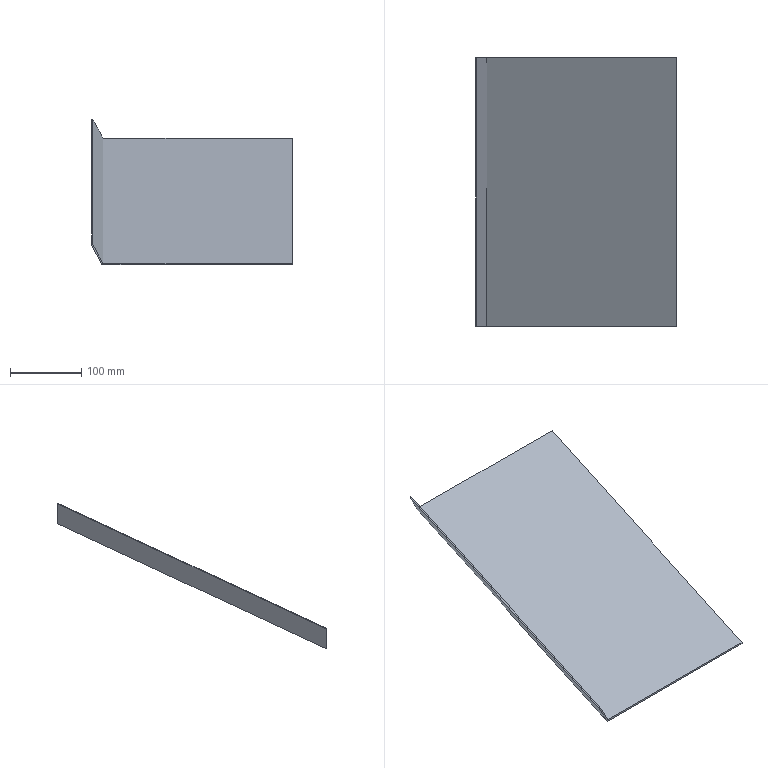Part | NX | features solid 2 | 1 solid | 8 faces | box 281.246 x 376.011 x 204.125 mm | volume 244430 mm3 | plane 8
STEP:
#1=CARTESIAN_POINT('',(748.754,-108.989,-45.166));
#2=VERTEX_POINT('',#1);
#3=CARTESIAN_POINT('',(763.321,-108.989,-73.005));
#4=VERTEX_POINT('',#3);
#5=CARTESIAN_POINT('',(693.858,-108.989,59.746));
#6=DIRECTION('',(0.4636,0.,-0.886));
#7=VECTOR('',#6,1000.);
#8=LINE('',#5,#7);
#9=EDGE_CURVE('',#2,#4,#8,.T.);
#10=ORIENTED_EDGE('',*,*,#9,.F.);
#11=CARTESIAN_POINT('',(750.567,-108.989,-44.218));
#12=VERTEX_POINT('',#11);
#13=CARTESIAN_POINT('',(876.733,-108.989,21.8));
#14=DIRECTION('',(0.886,0.,0.4636));
#15=VECTOR('',#14,1000.);
#16=LINE('',#13,#15);
#17=EDGE_CURVE('',#2,#12,#16,.T.);
#18=ORIENTED_EDGE('',*,*,#17,.T.);
#19=CARTESIAN_POINT('',(764.475,-108.989,-70.799));
#20=VERTEX_POINT('',#19);
#21=CARTESIAN_POINT('',(695.671,-108.989,60.694));
#22=DIRECTION('',(0.4636,0.,-0.886));
#23=VECTOR('',#22,1000.);
#24=LINE('',#21,#23);
#25=EDGE_CURVE('',#12,#20,#24,.T.);
#26=ORIENTED_EDGE('',*,*,#25,.T.);
#27=CARTESIAN_POINT('',(1030.,-108.989,-70.799));
#28=VERTEX_POINT('',#27);
#29=CARTESIAN_POINT('',(930.,-108.989,-70.799));
#30=DIRECTION('',(-1.,0.,0.));
#31=VECTOR('',#30,1000.);
#32=LINE('',#29,#31);
#33=EDGE_CURVE('',#28,#20,#32,.T.);
#34=ORIENTED_EDGE('',*,*,#33,.F.);
#35=CARTESIAN_POINT('',(1030.,-108.989,-73.005));
#36=VERTEX_POINT('',#35);
#37=CARTESIAN_POINT('',(1030.,-108.989,-80.));
#38=DIRECTION('',(0.,0.,1.));
#39=VECTOR('',#38,1000.);
#40=LINE('',#37,#39);
#41=EDGE_CURVE('',#36,#28,#40,.T.);
#42=ORIENTED_EDGE('',*,*,#41,.F.);
#43=CARTESIAN_POINT('',(930.,-108.989,-73.005));
#44=DIRECTION('',(-1.,0.,0.));
#45=VECTOR('',#44,1000.);
#46=LINE('',#43,#45);
#47=EDGE_CURVE('',#36,#4,#46,.T.);
#48=ORIENTED_EDGE('',*,*,#47,.T.);
#49=EDGE_LOOP('',(#10,#18,#26,#34,#42,#48));
#50=FACE_BOUND('',#49,.T.);
#51=CARTESIAN_POINT('',(930.,-108.989,-80.));
#52=DIRECTION('',(0.,-1.,0.));
#53=DIRECTION('',(0.,0.,-1.));
#54=AXIS2_PLACEMENT_3D('',#51,#52,#53);
#55=PLANE('',#54);
#56=ADVANCED_FACE('',(#50),#55,.F.);
#57=ORIENTED_EDGE('',*,*,#47,.F.);
#58=CARTESIAN_POINT('',(1030.,-485.,-248.342));
#59=VERTEX_POINT('',#58);
#60=CARTESIAN_POINT('',(1030.,-511.683,-260.785));
#61=DIRECTION('',(0.,0.9063,0.4226));
#62=VECTOR('',#61,1000.);
#63=LINE('',#60,#62);
#64=EDGE_CURVE('',#59,#36,#63,.T.);
#65=ORIENTED_EDGE('',*,*,#64,.F.);
#66=CARTESIAN_POINT('',(763.321,-485.,-248.342));
#67=VERTEX_POINT('',#66);
#68=CARTESIAN_POINT('',(930.,-485.,-248.342));
#69=DIRECTION('',(1.,0.,0.));
#70=VECTOR('',#69,1000.);
#71=LINE('',#68,#70);
#72=EDGE_CURVE('',#59,#67,#71,.F.);
#73=ORIENTED_EDGE('',*,*,#72,.T.);
#74=CARTESIAN_POINT('',(763.321,-81.099,-60.));
#75=DIRECTION('',(0.,0.9063,0.4226));
#76=VECTOR('',#75,1000.);
#77=LINE('',#74,#76);
#78=EDGE_CURVE('',#4,#67,#77,.F.);
#79=ORIENTED_EDGE('',*,*,#78,.F.);
#80=EDGE_LOOP('',(#57,#65,#73,#79));
#81=FACE_BOUND('',#80,.T.);
#82=CARTESIAN_POINT('',(930.,-619.13,-310.888));
#83=DIRECTION('',(0.,0.4226,-0.9063));
#84=DIRECTION('',(1.,0.,0.));
#85=AXIS2_PLACEMENT_3D('',#82,#83,#84);
#86=PLANE('',#85);
#87=ADVANCED_FACE('',(#81),#86,.T.);
#88=CARTESIAN_POINT('',(1030.,-485.,-246.136));
#89=VERTEX_POINT('',#88);
#90=CARTESIAN_POINT('',(1030.,-512.528,-258.972));
#91=DIRECTION('',(0.,0.9063,0.4226));
#92=VECTOR('',#91,1000.);
#93=LINE('',#90,#92);
#94=EDGE_CURVE('',#89,#28,#93,.T.);
#95=ORIENTED_EDGE('',*,*,#94,.T.);
#96=ORIENTED_EDGE('',*,*,#33,.T.);
#97=CARTESIAN_POINT('',(764.475,-485.,-246.136));
#98=VERTEX_POINT('',#97);
#99=CARTESIAN_POINT('',(764.475,-619.975,-309.076));
#100=DIRECTION('',(0.,-0.9063,-0.4226));
#101=VECTOR('',#100,1000.);
#102=LINE('',#99,#101);
#103=EDGE_CURVE('',#20,#98,#102,.T.);
#104=ORIENTED_EDGE('',*,*,#103,.T.);
#105=CARTESIAN_POINT('',(930.,-485.,-246.136));
#106=DIRECTION('',(1.,0.,0.));
#107=VECTOR('',#106,1000.);
#108=LINE('',#105,#107);
#109=EDGE_CURVE('',#89,#98,#108,.F.);
#110=ORIENTED_EDGE('',*,*,#109,.F.);
#111=EDGE_LOOP('',(#95,#96,#104,#110));
#112=FACE_BOUND('',#111,.T.);
#113=CARTESIAN_POINT('',(930.,-619.975,-309.076));
#114=DIRECTION('',(0.,0.4226,-0.9063));
#115=DIRECTION('',(1.,0.,0.));
#116=AXIS2_PLACEMENT_3D('',#113,#114,#115);
#117=PLANE('',#116);
#118=ADVANCED_FACE('',(#112),#117,.F.);
#119=CARTESIAN_POINT('',(750.567,-485.,-219.555));
#120=VERTEX_POINT('',#119);
#121=CARTESIAN_POINT('',(750.567,-92.125,-36.354));
#122=DIRECTION('',(0.,0.9063,0.4226));
#123=VECTOR('',#122,1000.);
#124=LINE('',#121,#123);
#125=EDGE_CURVE('',#120,#12,#124,.T.);
#126=ORIENTED_EDGE('',*,*,#125,.F.);
#127=CARTESIAN_POINT('',(623.645,-485.,23.006));
#128=DIRECTION('',(-0.4636,0.,0.886));
#129=VECTOR('',#128,1000.);
#130=LINE('',#127,#129);
#131=EDGE_CURVE('',#120,#98,#130,.F.);
#132=ORIENTED_EDGE('',*,*,#131,.T.);
#133=ORIENTED_EDGE('',*,*,#103,.F.);
#134=ORIENTED_EDGE('',*,*,#25,.F.);
#135=EDGE_LOOP('',(#126,#132,#133,#134));
#136=FACE_BOUND('',#135,.T.);
#137=CARTESIAN_POINT('',(690.475,-136.111,57.976));
#138=DIRECTION('',(0.866,-0.2113,0.4532));
#139=DIRECTION('',(0.4532,-0.05132,-0.89));
#140=AXIS2_PLACEMENT_3D('',#137,#138,#139);
#141=PLANE('',#140);
#142=ADVANCED_FACE('',(#136),#141,.T.);
#143=CARTESIAN_POINT('',(748.754,-485.,-220.503));
#144=VERTEX_POINT('',#143);
#145=CARTESIAN_POINT('',(763.357,-485.,-212.862));
#146=DIRECTION('',(-0.886,0.,-0.4636));
#147=VECTOR('',#146,1000.);
#148=LINE('',#145,#147);
#149=EDGE_CURVE('',#144,#120,#148,.F.);
#150=ORIENTED_EDGE('',*,*,#149,.F.);
#151=CARTESIAN_POINT('',(621.832,-485.,22.058));
#152=DIRECTION('',(-0.4636,0.,0.886));
#153=VECTOR('',#152,1000.);
#154=LINE('',#151,#153);
#155=EDGE_CURVE('',#144,#67,#154,.F.);
#156=ORIENTED_EDGE('',*,*,#155,.T.);
#157=ORIENTED_EDGE('',*,*,#72,.F.);
#158=CARTESIAN_POINT('',(1030.,-485.,-75.));
#159=DIRECTION('',(0.,0.,-1.));
#160=VECTOR('',#159,1000.);
#161=LINE('',#158,#160);
#162=EDGE_CURVE('',#59,#89,#161,.F.);
#163=ORIENTED_EDGE('',*,*,#162,.T.);
#164=ORIENTED_EDGE('',*,*,#109,.T.);
#165=ORIENTED_EDGE('',*,*,#131,.F.);
#166=EDGE_LOOP('',(#150,#156,#157,#163,#164,#165));
#167=FACE_BOUND('',#166,.T.);
#168=CARTESIAN_POINT('',(691.22,-485.,-75.));
#169=DIRECTION('',(0.,1.,0.));
#170=DIRECTION('',(-1.,0.,0.));
#171=AXIS2_PLACEMENT_3D('',#168,#169,#170);
#172=PLANE('',#171);
#173=ADVANCED_FACE('',(#167),#172,.F.);
#174=ORIENTED_EDGE('',*,*,#64,.T.);
#175=ORIENTED_EDGE('',*,*,#41,.T.);
#176=ORIENTED_EDGE('',*,*,#94,.F.);
#177=ORIENTED_EDGE('',*,*,#162,.F.);
#178=EDGE_LOOP('',(#174,#175,#176,#177));
#179=FACE_BOUND('',#178,.T.);
#180=CARTESIAN_POINT('',(1030.,-575.,-125.));
#181=DIRECTION('',(1.,0.,0.));
#182=DIRECTION('',(0.,0.,-1.));
#183=AXIS2_PLACEMENT_3D('',#180,#181,#182);
#184=PLANE('',#183);
#185=ADVANCED_FACE('',(#179),#184,.T.);
#186=ORIENTED_EDGE('',*,*,#155,.F.);
#187=CARTESIAN_POINT('',(748.754,-91.761,-37.133));
#188=DIRECTION('',(0.,0.9063,0.4226));
#189=VECTOR('',#188,1000.);
#190=LINE('',#187,#189);
#191=EDGE_CURVE('',#144,#2,#190,.T.);
#192=ORIENTED_EDGE('',*,*,#191,.T.);
#193=ORIENTED_EDGE('',*,*,#9,.T.);
#194=ORIENTED_EDGE('',*,*,#78,.T.);
#195=EDGE_LOOP('',(#186,#192,#193,#194));
#196=FACE_BOUND('',#195,.T.);
#197=CARTESIAN_POINT('',(688.743,-135.689,57.069));
#198=DIRECTION('',(0.866,-0.2113,0.4532));
#199=DIRECTION('',(0.4532,-0.05132,-0.89));
#200=AXIS2_PLACEMENT_3D('',#197,#198,#199);
#201=PLANE('',#200);
#202=ADVANCED_FACE('',(#196),#201,.F.);
#203=ORIENTED_EDGE('',*,*,#17,.F.);
#204=ORIENTED_EDGE('',*,*,#191,.F.);
#205=ORIENTED_EDGE('',*,*,#149,.T.);
#206=ORIENTED_EDGE('',*,*,#125,.T.);
#207=EDGE_LOOP('',(#203,#204,#205,#206));
#208=FACE_BOUND('',#207,.T.);
#209=CARTESIAN_POINT('',(750.567,-485.,-219.555));
#210=DIRECTION('',(0.4285,0.3819,-0.8189));
#211=DIRECTION('',(-0.886,0.,-0.4636));
#212=AXIS2_PLACEMENT_3D('',#209,#210,#211);
#213=PLANE('',#212);
#214=ADVANCED_FACE('',(#208),#213,.F.);
#215=CLOSED_SHELL('',(#56,#87,#118,#142,#173,#185,#202,#214));
#216=MANIFOLD_SOLID_BREP('',#215);
#217=(LENGTH_UNIT()NAMED_UNIT(*)SI_UNIT(.MILLI.,.METRE.));
#218=UNCERTAINTY_MEASURE_WITH_UNIT(LENGTH_MEASURE(0.00001),#217,'','');
#219=(NAMED_UNIT(*)PLANE_ANGLE_UNIT()SI_UNIT($,.RADIAN.));
#220=(NAMED_UNIT(*)SI_UNIT($,.STERADIAN.)SOLID_ANGLE_UNIT());
#221=(GEOMETRIC_REPRESENTATION_CONTEXT(3)GLOBAL_UNCERTAINTY_ASSIGNED_CONTEXT((#218))GLOBAL_UNIT_ASSIGNED_CONTEXT((#217,#219,#220))REPRESENTATION_CONTEXT('',''));
#222=ADVANCED_BREP_SHAPE_REPRESENTATION('',(#216),#221);